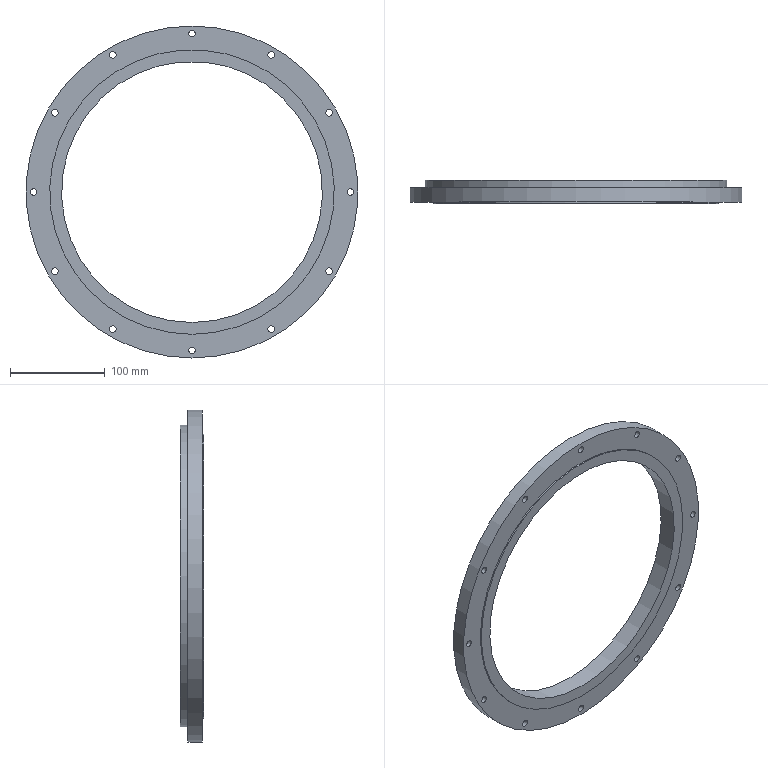Part | STEP file | Part [24] | 1 solid | 48 faces | box 350 x 24.5 x 350 mm | volume 570705 mm3 | cylinder 30 | plane 18 | commonest cylinder face diameters 7 x12 12 x12 275 x1 290 x1 300 x1 310 x1
STEP:
#1=CARTESIAN_POINT('',(0.,16.5,-175.));
#2=VERTEX_POINT('',#1);
#3=CARTESIAN_POINT('',(0.,16.5,0.));
#4=DIRECTION('',(0.,-1.,0.));
#5=DIRECTION('',(0.,0.,-1.));
#6=AXIS2_PLACEMENT_3D('',#3,#4,#5);
#7=CIRCLE('',#6,175.);
#8=EDGE_CURVE('',#2,#2,#7,.T.);
#9=ORIENTED_EDGE('',*,*,#8,.F.);
#10=EDGE_LOOP('',(#9));
#11=FACE_BOUND('',#10,.T.);
#12=CARTESIAN_POINT('',(88.696,16.5,141.626));
#13=VERTEX_POINT('',#12);
#14=CARTESIAN_POINT('',(83.5,16.5,144.626));
#15=DIRECTION('',(0.,1.,0.));
#16=DIRECTION('',(0.866,0.,-0.5));
#17=AXIS2_PLACEMENT_3D('',#14,#15,#16);
#18=CIRCLE('',#17,6.);
#19=EDGE_CURVE('',#13,#13,#18,.F.);
#20=ORIENTED_EDGE('',*,*,#19,.T.);
#21=EDGE_LOOP('',(#20));
#22=FACE_BOUND('',#21,.T.);
#23=CARTESIAN_POINT('',(147.626,16.5,78.304));
#24=VERTEX_POINT('',#23);
#25=CARTESIAN_POINT('',(144.626,16.5,83.5));
#26=DIRECTION('',(0.,1.,0.));
#27=DIRECTION('',(0.5,0.,-0.866));
#28=AXIS2_PLACEMENT_3D('',#25,#26,#27);
#29=CIRCLE('',#28,6.);
#30=EDGE_CURVE('',#24,#24,#29,.F.);
#31=ORIENTED_EDGE('',*,*,#30,.T.);
#32=EDGE_LOOP('',(#31));
#33=FACE_BOUND('',#32,.T.);
#34=CARTESIAN_POINT('',(167.,16.5,-6.));
#35=VERTEX_POINT('',#34);
#36=CARTESIAN_POINT('',(167.,16.5,0.));
#37=DIRECTION('',(0.,1.,0.));
#38=DIRECTION('',(0.,0.,-1.));
#39=AXIS2_PLACEMENT_3D('',#36,#37,#38);
#40=CIRCLE('',#39,6.);
#41=EDGE_CURVE('',#35,#35,#40,.F.);
#42=ORIENTED_EDGE('',*,*,#41,.T.);
#43=EDGE_LOOP('',(#42));
#44=FACE_BOUND('',#43,.T.);
#45=CARTESIAN_POINT('',(141.626,16.5,-88.696));
#46=VERTEX_POINT('',#45);
#47=CARTESIAN_POINT('',(144.626,16.5,-83.5));
#48=DIRECTION('',(0.,1.,0.));
#49=DIRECTION('',(-0.5,0.,-0.866));
#50=AXIS2_PLACEMENT_3D('',#47,#48,#49);
#51=CIRCLE('',#50,6.);
#52=EDGE_CURVE('',#46,#46,#51,.F.);
#53=ORIENTED_EDGE('',*,*,#52,.T.);
#54=EDGE_LOOP('',(#53));
#55=FACE_BOUND('',#54,.T.);
#56=CARTESIAN_POINT('',(78.304,16.5,-147.626));
#57=VERTEX_POINT('',#56);
#58=CARTESIAN_POINT('',(83.5,16.5,-144.626));
#59=DIRECTION('',(0.,1.,0.));
#60=DIRECTION('',(-0.866,0.,-0.5));
#61=AXIS2_PLACEMENT_3D('',#58,#59,#60);
#62=CIRCLE('',#61,6.);
#63=EDGE_CURVE('',#57,#57,#62,.F.);
#64=ORIENTED_EDGE('',*,*,#63,.T.);
#65=EDGE_LOOP('',(#64));
#66=FACE_BOUND('',#65,.T.);
#67=CARTESIAN_POINT('',(-6.,16.5,-167.));
#68=VERTEX_POINT('',#67);
#69=CARTESIAN_POINT('',(0.,16.5,-167.));
#70=DIRECTION('',(0.,1.,0.));
#71=DIRECTION('',(-1.,0.,0.));
#72=AXIS2_PLACEMENT_3D('',#69,#70,#71);
#73=CIRCLE('',#72,6.);
#74=EDGE_CURVE('',#68,#68,#73,.F.);
#75=ORIENTED_EDGE('',*,*,#74,.T.);
#76=EDGE_LOOP('',(#75));
#77=FACE_BOUND('',#76,.T.);
#78=CARTESIAN_POINT('',(-88.696,16.5,-141.626));
#79=VERTEX_POINT('',#78);
#80=CARTESIAN_POINT('',(-83.5,16.5,-144.626));
#81=DIRECTION('',(0.,1.,0.));
#82=DIRECTION('',(-0.866,0.,0.5));
#83=AXIS2_PLACEMENT_3D('',#80,#81,#82);
#84=CIRCLE('',#83,6.);
#85=EDGE_CURVE('',#79,#79,#84,.F.);
#86=ORIENTED_EDGE('',*,*,#85,.T.);
#87=EDGE_LOOP('',(#86));
#88=FACE_BOUND('',#87,.T.);
#89=CARTESIAN_POINT('',(-147.626,16.5,-78.304));
#90=VERTEX_POINT('',#89);
#91=CARTESIAN_POINT('',(-144.626,16.5,-83.5));
#92=DIRECTION('',(0.,1.,0.));
#93=DIRECTION('',(-0.5,0.,0.866));
#94=AXIS2_PLACEMENT_3D('',#91,#92,#93);
#95=CIRCLE('',#94,6.);
#96=EDGE_CURVE('',#90,#90,#95,.F.);
#97=ORIENTED_EDGE('',*,*,#96,.T.);
#98=EDGE_LOOP('',(#97));
#99=FACE_BOUND('',#98,.T.);
#100=CARTESIAN_POINT('',(-167.,16.5,6.));
#101=VERTEX_POINT('',#100);
#102=CARTESIAN_POINT('',(-167.,16.5,0.));
#103=DIRECTION('',(0.,1.,0.));
#104=DIRECTION('',(0.,0.,1.));
#105=AXIS2_PLACEMENT_3D('',#102,#103,#104);
#106=CIRCLE('',#105,6.);
#107=EDGE_CURVE('',#101,#101,#106,.F.);
#108=ORIENTED_EDGE('',*,*,#107,.T.);
#109=EDGE_LOOP('',(#108));
#110=FACE_BOUND('',#109,.T.);
#111=CARTESIAN_POINT('',(-141.626,16.5,88.696));
#112=VERTEX_POINT('',#111);
#113=CARTESIAN_POINT('',(-144.626,16.5,83.5));
#114=DIRECTION('',(0.,1.,0.));
#115=DIRECTION('',(0.5,0.,0.866));
#116=AXIS2_PLACEMENT_3D('',#113,#114,#115);
#117=CIRCLE('',#116,6.);
#118=EDGE_CURVE('',#112,#112,#117,.F.);
#119=ORIENTED_EDGE('',*,*,#118,.T.);
#120=EDGE_LOOP('',(#119));
#121=FACE_BOUND('',#120,.T.);
#122=CARTESIAN_POINT('',(-78.304,16.5,147.626));
#123=VERTEX_POINT('',#122);
#124=CARTESIAN_POINT('',(-83.5,16.5,144.626));
#125=DIRECTION('',(0.,1.,0.));
#126=DIRECTION('',(0.866,0.,0.5));
#127=AXIS2_PLACEMENT_3D('',#124,#125,#126);
#128=CIRCLE('',#127,6.);
#129=EDGE_CURVE('',#123,#123,#128,.F.);
#130=ORIENTED_EDGE('',*,*,#129,.T.);
#131=EDGE_LOOP('',(#130));
#132=FACE_BOUND('',#131,.T.);
#133=CARTESIAN_POINT('',(0.,16.5,-159.));
#134=VERTEX_POINT('',#133);
#135=CARTESIAN_POINT('',(0.,16.5,0.));
#136=DIRECTION('',(0.,-1.,0.));
#137=DIRECTION('',(0.,0.,-1.));
#138=AXIS2_PLACEMENT_3D('',#135,#136,#137);
#139=CIRCLE('',#138,159.);
#140=EDGE_CURVE('',#134,#134,#139,.T.);
#141=ORIENTED_EDGE('',*,*,#140,.T.);
#142=EDGE_LOOP('',(#141));
#143=FACE_BOUND('',#142,.T.);
#144=CARTESIAN_POINT('',(6.,16.5,167.));
#145=VERTEX_POINT('',#144);
#146=CARTESIAN_POINT('',(0.,16.5,167.));
#147=DIRECTION('',(0.,1.,0.));
#148=DIRECTION('',(1.,0.,0.));
#149=AXIS2_PLACEMENT_3D('',#146,#147,#148);
#150=CIRCLE('',#149,6.);
#151=EDGE_CURVE('',#145,#145,#150,.F.);
#152=ORIENTED_EDGE('',*,*,#151,.T.);
#153=EDGE_LOOP('',(#152));
#154=FACE_BOUND('',#153,.T.);
#155=CARTESIAN_POINT('',(0.,16.5,0.));
#156=DIRECTION('',(0.,1.,0.));
#157=DIRECTION('',(0.,0.,-1.));
#158=AXIS2_PLACEMENT_3D('',#155,#156,#157);
#159=PLANE('',#158);
#160=ADVANCED_FACE('',(#11,#22,#33,#44,#55,#66,#77,#88,#99,#110,#121,#132,#143,#154),#159,.T.);
#161=CARTESIAN_POINT('',(0.,1.5,-175.));
#162=VERTEX_POINT('',#161);
#163=CARTESIAN_POINT('',(0.,1.5,0.));
#164=DIRECTION('',(0.,-1.,0.));
#165=DIRECTION('',(0.,0.,-1.));
#166=AXIS2_PLACEMENT_3D('',#163,#164,#165);
#167=CIRCLE('',#166,175.);
#168=EDGE_CURVE('',#162,#162,#167,.T.);
#169=ORIENTED_EDGE('',*,*,#168,.T.);
#170=EDGE_LOOP('',(#169));
#171=FACE_BOUND('',#170,.T.);
#172=CARTESIAN_POINT('',(86.531,1.5,142.876));
#173=VERTEX_POINT('',#172);
#174=CARTESIAN_POINT('',(83.5,1.5,144.626));
#175=DIRECTION('',(0.,1.,0.));
#176=DIRECTION('',(0.866,0.,-0.5));
#177=AXIS2_PLACEMENT_3D('',#174,#175,#176);
#178=CIRCLE('',#177,3.5);
#179=EDGE_CURVE('',#173,#173,#178,.T.);
#180=ORIENTED_EDGE('',*,*,#179,.T.);
#181=EDGE_LOOP('',(#180));
#182=FACE_BOUND('',#181,.T.);
#183=CARTESIAN_POINT('',(146.376,1.5,80.469));
#184=VERTEX_POINT('',#183);
#185=CARTESIAN_POINT('',(144.626,1.5,83.5));
#186=DIRECTION('',(0.,1.,0.));
#187=DIRECTION('',(0.5,0.,-0.866));
#188=AXIS2_PLACEMENT_3D('',#185,#186,#187);
#189=CIRCLE('',#188,3.5);
#190=EDGE_CURVE('',#184,#184,#189,.T.);
#191=ORIENTED_EDGE('',*,*,#190,.T.);
#192=EDGE_LOOP('',(#191));
#193=FACE_BOUND('',#192,.T.);
#194=CARTESIAN_POINT('',(167.,1.5,-3.5));
#195=VERTEX_POINT('',#194);
#196=CARTESIAN_POINT('',(167.,1.5,0.));
#197=DIRECTION('',(0.,1.,0.));
#198=DIRECTION('',(0.,0.,-1.));
#199=AXIS2_PLACEMENT_3D('',#196,#197,#198);
#200=CIRCLE('',#199,3.5);
#201=EDGE_CURVE('',#195,#195,#200,.T.);
#202=ORIENTED_EDGE('',*,*,#201,.T.);
#203=EDGE_LOOP('',(#202));
#204=FACE_BOUND('',#203,.T.);
#205=CARTESIAN_POINT('',(142.876,1.5,-86.531));
#206=VERTEX_POINT('',#205);
#207=CARTESIAN_POINT('',(144.626,1.5,-83.5));
#208=DIRECTION('',(0.,1.,0.));
#209=DIRECTION('',(-0.5,0.,-0.866));
#210=AXIS2_PLACEMENT_3D('',#207,#208,#209);
#211=CIRCLE('',#210,3.5);
#212=EDGE_CURVE('',#206,#206,#211,.T.);
#213=ORIENTED_EDGE('',*,*,#212,.T.);
#214=EDGE_LOOP('',(#213));
#215=FACE_BOUND('',#214,.T.);
#216=CARTESIAN_POINT('',(80.469,1.5,-146.376));
#217=VERTEX_POINT('',#216);
#218=CARTESIAN_POINT('',(83.5,1.5,-144.626));
#219=DIRECTION('',(0.,1.,0.));
#220=DIRECTION('',(-0.866,0.,-0.5));
#221=AXIS2_PLACEMENT_3D('',#218,#219,#220);
#222=CIRCLE('',#221,3.5);
#223=EDGE_CURVE('',#217,#217,#222,.T.);
#224=ORIENTED_EDGE('',*,*,#223,.T.);
#225=EDGE_LOOP('',(#224));
#226=FACE_BOUND('',#225,.T.);
#227=CARTESIAN_POINT('',(-3.5,1.5,-167.));
#228=VERTEX_POINT('',#227);
#229=CARTESIAN_POINT('',(0.,1.5,-167.));
#230=DIRECTION('',(0.,1.,0.));
#231=DIRECTION('',(-1.,0.,0.));
#232=AXIS2_PLACEMENT_3D('',#229,#230,#231);
#233=CIRCLE('',#232,3.5);
#234=EDGE_CURVE('',#228,#228,#233,.T.);
#235=ORIENTED_EDGE('',*,*,#234,.T.);
#236=EDGE_LOOP('',(#235));
#237=FACE_BOUND('',#236,.T.);
#238=CARTESIAN_POINT('',(-86.531,1.5,-142.876));
#239=VERTEX_POINT('',#238);
#240=CARTESIAN_POINT('',(-83.5,1.5,-144.626));
#241=DIRECTION('',(0.,1.,0.));
#242=DIRECTION('',(-0.866,0.,0.5));
#243=AXIS2_PLACEMENT_3D('',#240,#241,#242);
#244=CIRCLE('',#243,3.5);
#245=EDGE_CURVE('',#239,#239,#244,.T.);
#246=ORIENTED_EDGE('',*,*,#245,.T.);
#247=EDGE_LOOP('',(#246));
#248=FACE_BOUND('',#247,.T.);
#249=CARTESIAN_POINT('',(-146.376,1.5,-80.469));
#250=VERTEX_POINT('',#249);
#251=CARTESIAN_POINT('',(-144.626,1.5,-83.5));
#252=DIRECTION('',(0.,1.,0.));
#253=DIRECTION('',(-0.5,0.,0.866));
#254=AXIS2_PLACEMENT_3D('',#251,#252,#253);
#255=CIRCLE('',#254,3.5);
#256=EDGE_CURVE('',#250,#250,#255,.T.);
#257=ORIENTED_EDGE('',*,*,#256,.T.);
#258=EDGE_LOOP('',(#257));
#259=FACE_BOUND('',#258,.T.);
#260=CARTESIAN_POINT('',(-167.,1.5,3.5));
#261=VERTEX_POINT('',#260);
#262=CARTESIAN_POINT('',(-167.,1.5,0.));
#263=DIRECTION('',(0.,1.,0.));
#264=DIRECTION('',(0.,0.,1.));
#265=AXIS2_PLACEMENT_3D('',#262,#263,#264);
#266=CIRCLE('',#265,3.5);
#267=EDGE_CURVE('',#261,#261,#266,.T.);
#268=ORIENTED_EDGE('',*,*,#267,.T.);
#269=EDGE_LOOP('',(#268));
#270=FACE_BOUND('',#269,.T.);
#271=CARTESIAN_POINT('',(-142.876,1.5,86.531));
#272=VERTEX_POINT('',#271);
#273=CARTESIAN_POINT('',(-144.626,1.5,83.5));
#274=DIRECTION('',(0.,1.,0.));
#275=DIRECTION('',(0.5,0.,0.866));
#276=AXIS2_PLACEMENT_3D('',#273,#274,#275);
#277=CIRCLE('',#276,3.5);
#278=EDGE_CURVE('',#272,#272,#277,.T.);
#279=ORIENTED_EDGE('',*,*,#278,.T.);
#280=EDGE_LOOP('',(#279));
#281=FACE_BOUND('',#280,.T.);
#282=CARTESIAN_POINT('',(-80.469,1.5,146.376));
#283=VERTEX_POINT('',#282);
#284=CARTESIAN_POINT('',(-83.5,1.5,144.626));
#285=DIRECTION('',(0.,1.,0.));
#286=DIRECTION('',(0.866,0.,0.5));
#287=AXIS2_PLACEMENT_3D('',#284,#285,#286);
#288=CIRCLE('',#287,3.5);
#289=EDGE_CURVE('',#283,#283,#288,.T.);
#290=ORIENTED_EDGE('',*,*,#289,.T.);
#291=EDGE_LOOP('',(#290));
#292=FACE_BOUND('',#291,.T.);
#293=CARTESIAN_POINT('',(0.,1.5,-150.));
#294=VERTEX_POINT('',#293);
#295=CARTESIAN_POINT('',(0.,1.5,0.));
#296=DIRECTION('',(0.,-1.,0.));
#297=DIRECTION('',(0.,0.,-1.));
#298=AXIS2_PLACEMENT_3D('',#295,#296,#297);
#299=CIRCLE('',#298,150.);
#300=EDGE_CURVE('',#294,#294,#299,.T.);
#301=ORIENTED_EDGE('',*,*,#300,.F.);
#302=EDGE_LOOP('',(#301));
#303=FACE_BOUND('',#302,.T.);
#304=CARTESIAN_POINT('',(3.5,1.5,167.));
#305=VERTEX_POINT('',#304);
#306=CARTESIAN_POINT('',(0.,1.5,167.));
#307=DIRECTION('',(0.,1.,0.));
#308=DIRECTION('',(1.,0.,0.));
#309=AXIS2_PLACEMENT_3D('',#306,#307,#308);
#310=CIRCLE('',#309,3.5);
#311=EDGE_CURVE('',#305,#305,#310,.T.);
#312=ORIENTED_EDGE('',*,*,#311,.T.);
#313=EDGE_LOOP('',(#312));
#314=FACE_BOUND('',#313,.T.);
#315=CARTESIAN_POINT('',(0.,1.5,0.));
#316=DIRECTION('',(0.,-1.,0.));
#317=DIRECTION('',(0.,0.,-1.));
#318=AXIS2_PLACEMENT_3D('',#315,#316,#317);
#319=PLANE('',#318);
#320=ADVANCED_FACE('',(#171,#182,#193,#204,#215,#226,#237,#248,#259,#270,#281,#292,#303,#314),#319,.T.);
#321=CARTESIAN_POINT('',(-80.469,10.5,146.376));
#322=VERTEX_POINT('',#321);
#323=CARTESIAN_POINT('',(-83.5,10.5,144.626));
#324=DIRECTION('',(0.,1.,0.));
#325=DIRECTION('',(0.866,0.,0.5));
#326=AXIS2_PLACEMENT_3D('',#323,#324,#325);
#327=CIRCLE('',#326,3.5);
#328=EDGE_CURVE('',#322,#322,#327,.T.);
#329=ORIENTED_EDGE('',*,*,#328,.T.);
#330=EDGE_LOOP('',(#329));
#331=FACE_OUTER_BOUND('',#330,.T.);
#332=ORIENTED_EDGE('',*,*,#289,.F.);
#333=EDGE_LOOP('',(#332));
#334=FACE_OUTER_BOUND('',#333,.T.);
#335=CARTESIAN_POINT('',(-83.5,-23.5,144.626));
#336=DIRECTION('',(0.,1.,0.));
#337=DIRECTION('',(0.866,0.,0.5));
#338=AXIS2_PLACEMENT_3D('',#335,#336,#337);
#339=CYLINDRICAL_SURFACE('',#338,3.5);
#340=ADVANCED_FACE('',(#331,#334),#339,.F.);
#341=ORIENTED_EDGE('',*,*,#129,.F.);
#342=EDGE_LOOP('',(#341));
#343=FACE_OUTER_BOUND('',#342,.T.);
#344=CARTESIAN_POINT('',(-78.304,10.5,147.626));
#345=VERTEX_POINT('',#344);
#346=CARTESIAN_POINT('',(-83.5,10.5,144.626));
#347=DIRECTION('',(0.,1.,0.));
#348=DIRECTION('',(0.866,0.,0.5));
#349=AXIS2_PLACEMENT_3D('',#346,#347,#348);
#350=CIRCLE('',#349,6.);
#351=EDGE_CURVE('',#345,#345,#350,.T.);
#352=ORIENTED_EDGE('',*,*,#351,.F.);
#353=EDGE_LOOP('',(#352));
#354=FACE_OUTER_BOUND('',#353,.T.);
#355=CARTESIAN_POINT('',(-83.5,10.5,144.626));
#356=DIRECTION('',(0.,1.,0.));
#357=DIRECTION('',(0.866,0.,0.5));
#358=AXIS2_PLACEMENT_3D('',#355,#356,#357);
#359=CYLINDRICAL_SURFACE('',#358,6.);
#360=ADVANCED_FACE('',(#343,#354),#359,.F.);
#361=CARTESIAN_POINT('',(-142.876,10.5,86.531));
#362=VERTEX_POINT('',#361);
#363=CARTESIAN_POINT('',(-144.626,10.5,83.5));
#364=DIRECTION('',(0.,1.,0.));
#365=DIRECTION('',(0.5,0.,0.866));
#366=AXIS2_PLACEMENT_3D('',#363,#364,#365);
#367=CIRCLE('',#366,3.5);
#368=EDGE_CURVE('',#362,#362,#367,.T.);
#369=ORIENTED_EDGE('',*,*,#368,.T.);
#370=EDGE_LOOP('',(#369));
#371=FACE_OUTER_BOUND('',#370,.T.);
#372=ORIENTED_EDGE('',*,*,#278,.F.);
#373=EDGE_LOOP('',(#372));
#374=FACE_OUTER_BOUND('',#373,.T.);
#375=CARTESIAN_POINT('',(-144.626,-23.5,83.5));
#376=DIRECTION('',(0.,1.,0.));
#377=DIRECTION('',(0.5,0.,0.866));
#378=AXIS2_PLACEMENT_3D('',#375,#376,#377);
#379=CYLINDRICAL_SURFACE('',#378,3.5);
#380=ADVANCED_FACE('',(#371,#374),#379,.F.);
#381=ORIENTED_EDGE('',*,*,#118,.F.);
#382=EDGE_LOOP('',(#381));
#383=FACE_OUTER_BOUND('',#382,.T.);
#384=CARTESIAN_POINT('',(-141.626,10.5,88.696));
#385=VERTEX_POINT('',#384);
#386=CARTESIAN_POINT('',(-144.626,10.5,83.5));
#387=DIRECTION('',(0.,1.,0.));
#388=DIRECTION('',(0.5,0.,0.866));
#389=AXIS2_PLACEMENT_3D('',#386,#387,#388);
#390=CIRCLE('',#389,6.);
#391=EDGE_CURVE('',#385,#385,#390,.T.);
#392=ORIENTED_EDGE('',*,*,#391,.F.);
#393=EDGE_LOOP('',(#392));
#394=FACE_OUTER_BOUND('',#393,.T.);
#395=CARTESIAN_POINT('',(-144.626,10.5,83.5));
#396=DIRECTION('',(0.,1.,0.));
#397=DIRECTION('',(0.5,0.,0.866));
#398=AXIS2_PLACEMENT_3D('',#395,#396,#397);
#399=CYLINDRICAL_SURFACE('',#398,6.);
#400=ADVANCED_FACE('',(#383,#394),#399,.F.);
#401=CARTESIAN_POINT('',(-167.,10.5,3.5));
#402=VERTEX_POINT('',#401);
#403=CARTESIAN_POINT('',(-167.,10.5,0.));
#404=DIRECTION('',(0.,1.,0.));
#405=DIRECTION('',(0.,0.,1.));
#406=AXIS2_PLACEMENT_3D('',#403,#404,#405);
#407=CIRCLE('',#406,3.5);
#408=EDGE_CURVE('',#402,#402,#407,.T.);
#409=ORIENTED_EDGE('',*,*,#408,.T.);
#410=EDGE_LOOP('',(#409));
#411=FACE_OUTER_BOUND('',#410,.T.);
#412=ORIENTED_EDGE('',*,*,#267,.F.);
#413=EDGE_LOOP('',(#412));
#414=FACE_OUTER_BOUND('',#413,.T.);
#415=CARTESIAN_POINT('',(-167.,-23.5,0.));
#416=DIRECTION('',(0.,1.,0.));
#417=DIRECTION('',(0.,0.,1.));
#418=AXIS2_PLACEMENT_3D('',#415,#416,#417);
#419=CYLINDRICAL_SURFACE('',#418,3.5);
#420=ADVANCED_FACE('',(#411,#414),#419,.F.);
#421=ORIENTED_EDGE('',*,*,#107,.F.);
#422=EDGE_LOOP('',(#421));
#423=FACE_OUTER_BOUND('',#422,.T.);
#424=CARTESIAN_POINT('',(-167.,10.5,6.));
#425=VERTEX_POINT('',#424);
#426=CARTESIAN_POINT('',(-167.,10.5,0.));
#427=DIRECTION('',(0.,1.,0.));
#428=DIRECTION('',(0.,0.,1.));
#429=AXIS2_PLACEMENT_3D('',#426,#427,#428);
#430=CIRCLE('',#429,6.);
#431=EDGE_CURVE('',#425,#425,#430,.T.);
#432=ORIENTED_EDGE('',*,*,#431,.F.);
#433=EDGE_LOOP('',(#432));
#434=FACE_OUTER_BOUND('',#433,.T.);
#435=CARTESIAN_POINT('',(-167.,10.5,0.));
#436=DIRECTION('',(0.,1.,0.));
#437=DIRECTION('',(0.,0.,1.));
#438=AXIS2_PLACEMENT_3D('',#435,#436,#437);
#439=CYLINDRICAL_SURFACE('',#438,6.);
#440=ADVANCED_FACE('',(#423,#434),#439,.F.);
#441=CARTESIAN_POINT('',(-146.376,10.5,-80.469));
#442=VERTEX_POINT('',#441);
#443=CARTESIAN_POINT('',(-144.626,10.5,-83.5));
#444=DIRECTION('',(0.,1.,0.));
#445=DIRECTION('',(-0.5,0.,0.866));
#446=AXIS2_PLACEMENT_3D('',#443,#444,#445);
#447=CIRCLE('',#446,3.5);
#448=EDGE_CURVE('',#442,#442,#447,.T.);
#449=ORIENTED_EDGE('',*,*,#448,.T.);
#450=EDGE_LOOP('',(#449));
#451=FACE_OUTER_BOUND('',#450,.T.);
#452=ORIENTED_EDGE('',*,*,#256,.F.);
#453=EDGE_LOOP('',(#452));
#454=FACE_OUTER_BOUND('',#453,.T.);
#455=CARTESIAN_POINT('',(-144.626,-23.5,-83.5));
#456=DIRECTION('',(0.,1.,0.));
#457=DIRECTION('',(-0.5,0.,0.866));
#458=AXIS2_PLACEMENT_3D('',#455,#456,#457);
#459=CYLINDRICAL_SURFACE('',#458,3.5);
#460=ADVANCED_FACE('',(#451,#454),#459,.F.);
#461=ORIENTED_EDGE('',*,*,#96,.F.);
#462=EDGE_LOOP('',(#461));
#463=FACE_OUTER_BOUND('',#462,.T.);
#464=CARTESIAN_POINT('',(-147.626,10.5,-78.304));
#465=VERTEX_POINT('',#464);
#466=CARTESIAN_POINT('',(-144.626,10.5,-83.5));
#467=DIRECTION('',(0.,1.,0.));
#468=DIRECTION('',(-0.5,0.,0.866));
#469=AXIS2_PLACEMENT_3D('',#466,#467,#468);
#470=CIRCLE('',#469,6.);
#471=EDGE_CURVE('',#465,#465,#470,.T.);
#472=ORIENTED_EDGE('',*,*,#471,.F.);
#473=EDGE_LOOP('',(#472));
#474=FACE_OUTER_BOUND('',#473,.T.);
#475=CARTESIAN_POINT('',(-144.626,10.5,-83.5));
#476=DIRECTION('',(0.,1.,0.));
#477=DIRECTION('',(-0.5,0.,0.866));
#478=AXIS2_PLACEMENT_3D('',#475,#476,#477);
#479=CYLINDRICAL_SURFACE('',#478,6.);
#480=ADVANCED_FACE('',(#463,#474),#479,.F.);
#481=CARTESIAN_POINT('',(-86.531,10.5,-142.876));
#482=VERTEX_POINT('',#481);
#483=CARTESIAN_POINT('',(-83.5,10.5,-144.626));
#484=DIRECTION('',(0.,1.,0.));
#485=DIRECTION('',(-0.866,0.,0.5));
#486=AXIS2_PLACEMENT_3D('',#483,#484,#485);
#487=CIRCLE('',#486,3.5);
#488=EDGE_CURVE('',#482,#482,#487,.T.);
#489=ORIENTED_EDGE('',*,*,#488,.T.);
#490=EDGE_LOOP('',(#489));
#491=FACE_OUTER_BOUND('',#490,.T.);
#492=ORIENTED_EDGE('',*,*,#245,.F.);
#493=EDGE_LOOP('',(#492));
#494=FACE_OUTER_BOUND('',#493,.T.);
#495=CARTESIAN_POINT('',(-83.5,-23.5,-144.626));
#496=DIRECTION('',(0.,1.,0.));
#497=DIRECTION('',(-0.866,0.,0.5));
#498=AXIS2_PLACEMENT_3D('',#495,#496,#497);
#499=CYLINDRICAL_SURFACE('',#498,3.5);
#500=ADVANCED_FACE('',(#491,#494),#499,.F.);
#501=ORIENTED_EDGE('',*,*,#85,.F.);
#502=EDGE_LOOP('',(#501));
#503=FACE_OUTER_BOUND('',#502,.T.);
#504=CARTESIAN_POINT('',(-88.696,10.5,-141.626));
#505=VERTEX_POINT('',#504);
#506=CARTESIAN_POINT('',(-83.5,10.5,-144.626));
#507=DIRECTION('',(0.,1.,0.));
#508=DIRECTION('',(-0.866,0.,0.5));
#509=AXIS2_PLACEMENT_3D('',#506,#507,#508);
#510=CIRCLE('',#509,6.);
#511=EDGE_CURVE('',#505,#505,#510,.T.);
#512=ORIENTED_EDGE('',*,*,#511,.F.);
#513=EDGE_LOOP('',(#512));
#514=FACE_OUTER_BOUND('',#513,.T.);
#515=CARTESIAN_POINT('',(-83.5,10.5,-144.626));
#516=DIRECTION('',(0.,1.,0.));
#517=DIRECTION('',(-0.866,0.,0.5));
#518=AXIS2_PLACEMENT_3D('',#515,#516,#517);
#519=CYLINDRICAL_SURFACE('',#518,6.);
#520=ADVANCED_FACE('',(#503,#514),#519,.F.);
#521=CARTESIAN_POINT('',(-3.5,10.5,-167.));
#522=VERTEX_POINT('',#521);
#523=CARTESIAN_POINT('',(0.,10.5,-167.));
#524=DIRECTION('',(0.,1.,0.));
#525=DIRECTION('',(-1.,0.,0.));
#526=AXIS2_PLACEMENT_3D('',#523,#524,#525);
#527=CIRCLE('',#526,3.5);
#528=EDGE_CURVE('',#522,#522,#527,.T.);
#529=ORIENTED_EDGE('',*,*,#528,.T.);
#530=EDGE_LOOP('',(#529));
#531=FACE_OUTER_BOUND('',#530,.T.);
#532=ORIENTED_EDGE('',*,*,#234,.F.);
#533=EDGE_LOOP('',(#532));
#534=FACE_OUTER_BOUND('',#533,.T.);
#535=CARTESIAN_POINT('',(0.,-23.5,-167.));
#536=DIRECTION('',(0.,1.,0.));
#537=DIRECTION('',(-1.,0.,0.));
#538=AXIS2_PLACEMENT_3D('',#535,#536,#537);
#539=CYLINDRICAL_SURFACE('',#538,3.5);
#540=ADVANCED_FACE('',(#531,#534),#539,.F.);
#541=ORIENTED_EDGE('',*,*,#74,.F.);
#542=EDGE_LOOP('',(#541));
#543=FACE_OUTER_BOUND('',#542,.T.);
#544=CARTESIAN_POINT('',(-6.,10.5,-167.));
#545=VERTEX_POINT('',#544);
#546=CARTESIAN_POINT('',(0.,10.5,-167.));
#547=DIRECTION('',(0.,1.,0.));
#548=DIRECTION('',(-1.,0.,0.));
#549=AXIS2_PLACEMENT_3D('',#546,#547,#548);
#550=CIRCLE('',#549,6.);
#551=EDGE_CURVE('',#545,#545,#550,.T.);
#552=ORIENTED_EDGE('',*,*,#551,.F.);
#553=EDGE_LOOP('',(#552));
#554=FACE_OUTER_BOUND('',#553,.T.);
#555=CARTESIAN_POINT('',(0.,10.5,-167.));
#556=DIRECTION('',(0.,1.,0.));
#557=DIRECTION('',(-1.,0.,0.));
#558=AXIS2_PLACEMENT_3D('',#555,#556,#557);
#559=CYLINDRICAL_SURFACE('',#558,6.);
#560=ADVANCED_FACE('',(#543,#554),#559,.F.);
#561=CARTESIAN_POINT('',(80.469,10.5,-146.376));
#562=VERTEX_POINT('',#561);
#563=CARTESIAN_POINT('',(83.5,10.5,-144.626));
#564=DIRECTION('',(0.,1.,0.));
#565=DIRECTION('',(-0.866,0.,-0.5));
#566=AXIS2_PLACEMENT_3D('',#563,#564,#565);
#567=CIRCLE('',#566,3.5);
#568=EDGE_CURVE('',#562,#562,#567,.T.);
#569=ORIENTED_EDGE('',*,*,#568,.T.);
#570=EDGE_LOOP('',(#569));
#571=FACE_OUTER_BOUND('',#570,.T.);
#572=ORIENTED_EDGE('',*,*,#223,.F.);
#573=EDGE_LOOP('',(#572));
#574=FACE_OUTER_BOUND('',#573,.T.);
#575=CARTESIAN_POINT('',(83.5,-23.5,-144.626));
#576=DIRECTION('',(0.,1.,0.));
#577=DIRECTION('',(-0.866,0.,-0.5));
#578=AXIS2_PLACEMENT_3D('',#575,#576,#577);
#579=CYLINDRICAL_SURFACE('',#578,3.5);
#580=ADVANCED_FACE('',(#571,#574),#579,.F.);
#581=ORIENTED_EDGE('',*,*,#63,.F.);
#582=EDGE_LOOP('',(#581));
#583=FACE_OUTER_BOUND('',#582,.T.);
#584=CARTESIAN_POINT('',(78.304,10.5,-147.626));
#585=VERTEX_POINT('',#584);
#586=CARTESIAN_POINT('',(83.5,10.5,-144.626));
#587=DIRECTION('',(0.,1.,0.));
#588=DIRECTION('',(-0.866,0.,-0.5));
#589=AXIS2_PLACEMENT_3D('',#586,#587,#588);
#590=CIRCLE('',#589,6.);
#591=EDGE_CURVE('',#585,#585,#590,.T.);
#592=ORIENTED_EDGE('',*,*,#591,.F.);
#593=EDGE_LOOP('',(#592));
#594=FACE_OUTER_BOUND('',#593,.T.);
#595=CARTESIAN_POINT('',(83.5,10.5,-144.626));
#596=DIRECTION('',(0.,1.,0.));
#597=DIRECTION('',(-0.866,0.,-0.5));
#598=AXIS2_PLACEMENT_3D('',#595,#596,#597);
#599=CYLINDRICAL_SURFACE('',#598,6.);
#600=ADVANCED_FACE('',(#583,#594),#599,.F.);
#601=CARTESIAN_POINT('',(142.876,10.5,-86.531));
#602=VERTEX_POINT('',#601);
#603=CARTESIAN_POINT('',(144.626,10.5,-83.5));
#604=DIRECTION('',(0.,1.,0.));
#605=DIRECTION('',(-0.5,0.,-0.866));
#606=AXIS2_PLACEMENT_3D('',#603,#604,#605);
#607=CIRCLE('',#606,3.5);
#608=EDGE_CURVE('',#602,#602,#607,.T.);
#609=ORIENTED_EDGE('',*,*,#608,.T.);
#610=EDGE_LOOP('',(#609));
#611=FACE_OUTER_BOUND('',#610,.T.);
#612=ORIENTED_EDGE('',*,*,#212,.F.);
#613=EDGE_LOOP('',(#612));
#614=FACE_OUTER_BOUND('',#613,.T.);
#615=CARTESIAN_POINT('',(144.626,-23.5,-83.5));
#616=DIRECTION('',(0.,1.,0.));
#617=DIRECTION('',(-0.5,0.,-0.866));
#618=AXIS2_PLACEMENT_3D('',#615,#616,#617);
#619=CYLINDRICAL_SURFACE('',#618,3.5);
#620=ADVANCED_FACE('',(#611,#614),#619,.F.);
#621=ORIENTED_EDGE('',*,*,#52,.F.);
#622=EDGE_LOOP('',(#621));
#623=FACE_OUTER_BOUND('',#622,.T.);
#624=CARTESIAN_POINT('',(141.626,10.5,-88.696));
#625=VERTEX_POINT('',#624);
#626=CARTESIAN_POINT('',(144.626,10.5,-83.5));
#627=DIRECTION('',(0.,1.,0.));
#628=DIRECTION('',(-0.5,0.,-0.866));
#629=AXIS2_PLACEMENT_3D('',#626,#627,#628);
#630=CIRCLE('',#629,6.);
#631=EDGE_CURVE('',#625,#625,#630,.T.);
#632=ORIENTED_EDGE('',*,*,#631,.F.);
#633=EDGE_LOOP('',(#632));
#634=FACE_OUTER_BOUND('',#633,.T.);
#635=CARTESIAN_POINT('',(144.626,10.5,-83.5));
#636=DIRECTION('',(0.,1.,0.));
#637=DIRECTION('',(-0.5,0.,-0.866));
#638=AXIS2_PLACEMENT_3D('',#635,#636,#637);
#639=CYLINDRICAL_SURFACE('',#638,6.);
#640=ADVANCED_FACE('',(#623,#634),#639,.F.);
#641=CARTESIAN_POINT('',(167.,10.5,-3.5));
#642=VERTEX_POINT('',#641);
#643=CARTESIAN_POINT('',(167.,10.5,0.));
#644=DIRECTION('',(0.,1.,0.));
#645=DIRECTION('',(0.,0.,-1.));
#646=AXIS2_PLACEMENT_3D('',#643,#644,#645);
#647=CIRCLE('',#646,3.5);
#648=EDGE_CURVE('',#642,#642,#647,.T.);
#649=ORIENTED_EDGE('',*,*,#648,.T.);
#650=EDGE_LOOP('',(#649));
#651=FACE_OUTER_BOUND('',#650,.T.);
#652=ORIENTED_EDGE('',*,*,#201,.F.);
#653=EDGE_LOOP('',(#652));
#654=FACE_OUTER_BOUND('',#653,.T.);
#655=CARTESIAN_POINT('',(167.,-23.5,0.));
#656=DIRECTION('',(0.,1.,0.));
#657=DIRECTION('',(0.,0.,-1.));
#658=AXIS2_PLACEMENT_3D('',#655,#656,#657);
#659=CYLINDRICAL_SURFACE('',#658,3.5);
#660=ADVANCED_FACE('',(#651,#654),#659,.F.);
#661=ORIENTED_EDGE('',*,*,#41,.F.);
#662=EDGE_LOOP('',(#661));
#663=FACE_OUTER_BOUND('',#662,.T.);
#664=CARTESIAN_POINT('',(167.,10.5,-6.));
#665=VERTEX_POINT('',#664);
#666=CARTESIAN_POINT('',(167.,10.5,0.));
#667=DIRECTION('',(0.,1.,0.));
#668=DIRECTION('',(0.,0.,-1.));
#669=AXIS2_PLACEMENT_3D('',#666,#667,#668);
#670=CIRCLE('',#669,6.);
#671=EDGE_CURVE('',#665,#665,#670,.T.);
#672=ORIENTED_EDGE('',*,*,#671,.F.);
#673=EDGE_LOOP('',(#672));
#674=FACE_OUTER_BOUND('',#673,.T.);
#675=CARTESIAN_POINT('',(167.,10.5,0.));
#676=DIRECTION('',(0.,1.,0.));
#677=DIRECTION('',(0.,0.,-1.));
#678=AXIS2_PLACEMENT_3D('',#675,#676,#677);
#679=CYLINDRICAL_SURFACE('',#678,6.);
#680=ADVANCED_FACE('',(#663,#674),#679,.F.);
#681=CARTESIAN_POINT('',(146.376,10.5,80.469));
#682=VERTEX_POINT('',#681);
#683=CARTESIAN_POINT('',(144.626,10.5,83.5));
#684=DIRECTION('',(0.,1.,0.));
#685=DIRECTION('',(0.5,0.,-0.866));
#686=AXIS2_PLACEMENT_3D('',#683,#684,#685);
#687=CIRCLE('',#686,3.5);
#688=EDGE_CURVE('',#682,#682,#687,.T.);
#689=ORIENTED_EDGE('',*,*,#688,.T.);
#690=EDGE_LOOP('',(#689));
#691=FACE_OUTER_BOUND('',#690,.T.);
#692=ORIENTED_EDGE('',*,*,#190,.F.);
#693=EDGE_LOOP('',(#692));
#694=FACE_OUTER_BOUND('',#693,.T.);
#695=CARTESIAN_POINT('',(144.626,-23.5,83.5));
#696=DIRECTION('',(0.,1.,0.));
#697=DIRECTION('',(0.5,0.,-0.866));
#698=AXIS2_PLACEMENT_3D('',#695,#696,#697);
#699=CYLINDRICAL_SURFACE('',#698,3.5);
#700=ADVANCED_FACE('',(#691,#694),#699,.F.);
#701=ORIENTED_EDGE('',*,*,#30,.F.);
#702=EDGE_LOOP('',(#701));
#703=FACE_OUTER_BOUND('',#702,.T.);
#704=CARTESIAN_POINT('',(147.626,10.5,78.304));
#705=VERTEX_POINT('',#704);
#706=CARTESIAN_POINT('',(144.626,10.5,83.5));
#707=DIRECTION('',(0.,1.,0.));
#708=DIRECTION('',(0.5,0.,-0.866));
#709=AXIS2_PLACEMENT_3D('',#706,#707,#708);
#710=CIRCLE('',#709,6.);
#711=EDGE_CURVE('',#705,#705,#710,.T.);
#712=ORIENTED_EDGE('',*,*,#711,.F.);
#713=EDGE_LOOP('',(#712));
#714=FACE_OUTER_BOUND('',#713,.T.);
#715=CARTESIAN_POINT('',(144.626,10.5,83.5));
#716=DIRECTION('',(0.,1.,0.));
#717=DIRECTION('',(0.5,0.,-0.866));
#718=AXIS2_PLACEMENT_3D('',#715,#716,#717);
#719=CYLINDRICAL_SURFACE('',#718,6.);
#720=ADVANCED_FACE('',(#703,#714),#719,.F.);
#721=CARTESIAN_POINT('',(86.531,10.5,142.876));
#722=VERTEX_POINT('',#721);
#723=CARTESIAN_POINT('',(83.5,10.5,144.626));
#724=DIRECTION('',(0.,1.,0.));
#725=DIRECTION('',(0.866,0.,-0.5));
#726=AXIS2_PLACEMENT_3D('',#723,#724,#725);
#727=CIRCLE('',#726,3.5);
#728=EDGE_CURVE('',#722,#722,#727,.T.);
#729=ORIENTED_EDGE('',*,*,#728,.T.);
#730=EDGE_LOOP('',(#729));
#731=FACE_OUTER_BOUND('',#730,.T.);
#732=ORIENTED_EDGE('',*,*,#179,.F.);
#733=EDGE_LOOP('',(#732));
#734=FACE_OUTER_BOUND('',#733,.T.);
#735=CARTESIAN_POINT('',(83.5,-23.5,144.626));
#736=DIRECTION('',(0.,1.,0.));
#737=DIRECTION('',(0.866,0.,-0.5));
#738=AXIS2_PLACEMENT_3D('',#735,#736,#737);
#739=CYLINDRICAL_SURFACE('',#738,3.5);
#740=ADVANCED_FACE('',(#731,#734),#739,.F.);
#741=ORIENTED_EDGE('',*,*,#19,.F.);
#742=EDGE_LOOP('',(#741));
#743=FACE_OUTER_BOUND('',#742,.T.);
#744=CARTESIAN_POINT('',(88.696,10.5,141.626));
#745=VERTEX_POINT('',#744);
#746=CARTESIAN_POINT('',(83.5,10.5,144.626));
#747=DIRECTION('',(0.,1.,0.));
#748=DIRECTION('',(0.866,0.,-0.5));
#749=AXIS2_PLACEMENT_3D('',#746,#747,#748);
#750=CIRCLE('',#749,6.);
#751=EDGE_CURVE('',#745,#745,#750,.T.);
#752=ORIENTED_EDGE('',*,*,#751,.F.);
#753=EDGE_LOOP('',(#752));
#754=FACE_OUTER_BOUND('',#753,.T.);
#755=CARTESIAN_POINT('',(83.5,10.5,144.626));
#756=DIRECTION('',(0.,1.,0.));
#757=DIRECTION('',(0.866,0.,-0.5));
#758=AXIS2_PLACEMENT_3D('',#755,#756,#757);
#759=CYLINDRICAL_SURFACE('',#758,6.);
#760=ADVANCED_FACE('',(#743,#754),#759,.F.);
#761=ORIENTED_EDGE('',*,*,#8,.T.);
#762=EDGE_LOOP('',(#761));
#763=FACE_OUTER_BOUND('',#762,.T.);
#764=ORIENTED_EDGE('',*,*,#168,.F.);
#765=EDGE_LOOP('',(#764));
#766=FACE_OUTER_BOUND('',#765,.T.);
#767=CARTESIAN_POINT('',(0.,16.5,0.));
#768=DIRECTION('',(0.,-1.,0.));
#769=DIRECTION('',(0.,0.,-1.));
#770=AXIS2_PLACEMENT_3D('',#767,#768,#769);
#771=CYLINDRICAL_SURFACE('',#770,175.);
#772=ADVANCED_FACE('',(#763,#766),#771,.T.);
#773=CARTESIAN_POINT('',(0.,24.5,-159.));
#774=VERTEX_POINT('',#773);
#775=CARTESIAN_POINT('',(0.,24.5,0.));
#776=DIRECTION('',(0.,-1.,0.));
#777=DIRECTION('',(0.,0.,-1.));
#778=AXIS2_PLACEMENT_3D('',#775,#776,#777);
#779=CIRCLE('',#778,159.);
#780=EDGE_CURVE('',#774,#774,#779,.T.);
#781=ORIENTED_EDGE('',*,*,#780,.T.);
#782=EDGE_LOOP('',(#781));
#783=FACE_OUTER_BOUND('',#782,.T.);
#784=ORIENTED_EDGE('',*,*,#140,.F.);
#785=EDGE_LOOP('',(#784));
#786=FACE_OUTER_BOUND('',#785,.T.);
#787=CARTESIAN_POINT('',(0.,24.5,0.));
#788=DIRECTION('',(0.,-1.,0.));
#789=DIRECTION('',(0.,0.,-1.));
#790=AXIS2_PLACEMENT_3D('',#787,#788,#789);
#791=CYLINDRICAL_SURFACE('',#790,159.);
#792=ADVANCED_FACE('',(#783,#786),#791,.T.);
#793=ORIENTED_EDGE('',*,*,#151,.F.);
#794=EDGE_LOOP('',(#793));
#795=FACE_OUTER_BOUND('',#794,.T.);
#796=CARTESIAN_POINT('',(6.,10.5,167.));
#797=VERTEX_POINT('',#796);
#798=CARTESIAN_POINT('',(0.,10.5,167.));
#799=DIRECTION('',(0.,1.,0.));
#800=DIRECTION('',(1.,0.,0.));
#801=AXIS2_PLACEMENT_3D('',#798,#799,#800);
#802=CIRCLE('',#801,6.);
#803=EDGE_CURVE('',#797,#797,#802,.T.);
#804=ORIENTED_EDGE('',*,*,#803,.F.);
#805=EDGE_LOOP('',(#804));
#806=FACE_OUTER_BOUND('',#805,.T.);
#807=CARTESIAN_POINT('',(0.,10.5,167.));
#808=DIRECTION('',(0.,1.,0.));
#809=DIRECTION('',(1.,0.,0.));
#810=AXIS2_PLACEMENT_3D('',#807,#808,#809);
#811=CYLINDRICAL_SURFACE('',#810,6.);
#812=ADVANCED_FACE('',(#795,#806),#811,.F.);
#813=ORIENTED_EDGE('',*,*,#300,.T.);
#814=EDGE_LOOP('',(#813));
#815=FACE_OUTER_BOUND('',#814,.T.);
#816=CARTESIAN_POINT('',(0.,0.,-150.));
#817=VERTEX_POINT('',#816);
#818=CARTESIAN_POINT('',(0.,0.,0.));
#819=DIRECTION('',(0.,-1.,0.));
#820=DIRECTION('',(0.,0.,-1.));
#821=AXIS2_PLACEMENT_3D('',#818,#819,#820);
#822=CIRCLE('',#821,150.);
#823=EDGE_CURVE('',#817,#817,#822,.T.);
#824=ORIENTED_EDGE('',*,*,#823,.F.);
#825=EDGE_LOOP('',(#824));
#826=FACE_OUTER_BOUND('',#825,.T.);
#827=CARTESIAN_POINT('',(0.,1.5,0.));
#828=DIRECTION('',(0.,-1.,0.));
#829=DIRECTION('',(0.,0.,-1.));
#830=AXIS2_PLACEMENT_3D('',#827,#828,#829);
#831=CYLINDRICAL_SURFACE('',#830,150.);
#832=ADVANCED_FACE('',(#815,#826),#831,.T.);
#833=CARTESIAN_POINT('',(3.5,10.5,167.));
#834=VERTEX_POINT('',#833);
#835=CARTESIAN_POINT('',(0.,10.5,167.));
#836=DIRECTION('',(0.,1.,0.));
#837=DIRECTION('',(1.,0.,0.));
#838=AXIS2_PLACEMENT_3D('',#835,#836,#837);
#839=CIRCLE('',#838,3.5);
#840=EDGE_CURVE('',#834,#834,#839,.T.);
#841=ORIENTED_EDGE('',*,*,#840,.T.);
#842=EDGE_LOOP('',(#841));
#843=FACE_OUTER_BOUND('',#842,.T.);
#844=ORIENTED_EDGE('',*,*,#311,.F.);
#845=EDGE_LOOP('',(#844));
#846=FACE_OUTER_BOUND('',#845,.T.);
#847=CARTESIAN_POINT('',(0.,-23.5,167.));
#848=DIRECTION('',(0.,1.,0.));
#849=DIRECTION('',(1.,0.,0.));
#850=AXIS2_PLACEMENT_3D('',#847,#848,#849);
#851=CYLINDRICAL_SURFACE('',#850,3.5);
#852=ADVANCED_FACE('',(#843,#846),#851,.F.);
#853=ORIENTED_EDGE('',*,*,#351,.T.);
#854=EDGE_LOOP('',(#853));
#855=FACE_BOUND('',#854,.T.);
#856=ORIENTED_EDGE('',*,*,#328,.F.);
#857=EDGE_LOOP('',(#856));
#858=FACE_BOUND('',#857,.T.);
#859=CARTESIAN_POINT('',(-83.5,10.5,144.626));
#860=DIRECTION('',(0.,-1.,0.));
#861=DIRECTION('',(0.866,0.,0.5));
#862=AXIS2_PLACEMENT_3D('',#859,#860,#861);
#863=PLANE('',#862);
#864=ADVANCED_FACE('',(#855,#858),#863,.F.);
#865=ORIENTED_EDGE('',*,*,#391,.T.);
#866=EDGE_LOOP('',(#865));
#867=FACE_BOUND('',#866,.T.);
#868=ORIENTED_EDGE('',*,*,#368,.F.);
#869=EDGE_LOOP('',(#868));
#870=FACE_BOUND('',#869,.T.);
#871=CARTESIAN_POINT('',(-144.626,10.5,83.5));
#872=DIRECTION('',(0.,-1.,0.));
#873=DIRECTION('',(0.5,0.,0.866));
#874=AXIS2_PLACEMENT_3D('',#871,#872,#873);
#875=PLANE('',#874);
#876=ADVANCED_FACE('',(#867,#870),#875,.F.);
#877=ORIENTED_EDGE('',*,*,#431,.T.);
#878=EDGE_LOOP('',(#877));
#879=FACE_BOUND('',#878,.T.);
#880=ORIENTED_EDGE('',*,*,#408,.F.);
#881=EDGE_LOOP('',(#880));
#882=FACE_BOUND('',#881,.T.);
#883=CARTESIAN_POINT('',(-167.,10.5,0.));
#884=DIRECTION('',(0.,-1.,0.));
#885=DIRECTION('',(0.,0.,1.));
#886=AXIS2_PLACEMENT_3D('',#883,#884,#885);
#887=PLANE('',#886);
#888=ADVANCED_FACE('',(#879,#882),#887,.F.);
#889=ORIENTED_EDGE('',*,*,#471,.T.);
#890=EDGE_LOOP('',(#889));
#891=FACE_BOUND('',#890,.T.);
#892=ORIENTED_EDGE('',*,*,#448,.F.);
#893=EDGE_LOOP('',(#892));
#894=FACE_BOUND('',#893,.T.);
#895=CARTESIAN_POINT('',(-144.626,10.5,-83.5));
#896=DIRECTION('',(0.,-1.,0.));
#897=DIRECTION('',(-0.5,0.,0.866));
#898=AXIS2_PLACEMENT_3D('',#895,#896,#897);
#899=PLANE('',#898);
#900=ADVANCED_FACE('',(#891,#894),#899,.F.);
#901=ORIENTED_EDGE('',*,*,#511,.T.);
#902=EDGE_LOOP('',(#901));
#903=FACE_BOUND('',#902,.T.);
#904=ORIENTED_EDGE('',*,*,#488,.F.);
#905=EDGE_LOOP('',(#904));
#906=FACE_BOUND('',#905,.T.);
#907=CARTESIAN_POINT('',(-83.5,10.5,-144.626));
#908=DIRECTION('',(0.,-1.,0.));
#909=DIRECTION('',(-0.866,0.,0.5));
#910=AXIS2_PLACEMENT_3D('',#907,#908,#909);
#911=PLANE('',#910);
#912=ADVANCED_FACE('',(#903,#906),#911,.F.);
#913=ORIENTED_EDGE('',*,*,#551,.T.);
#914=EDGE_LOOP('',(#913));
#915=FACE_BOUND('',#914,.T.);
#916=ORIENTED_EDGE('',*,*,#528,.F.);
#917=EDGE_LOOP('',(#916));
#918=FACE_BOUND('',#917,.T.);
#919=CARTESIAN_POINT('',(0.,10.5,-167.));
#920=DIRECTION('',(0.,-1.,0.));
#921=DIRECTION('',(-1.,0.,0.));
#922=AXIS2_PLACEMENT_3D('',#919,#920,#921);
#923=PLANE('',#922);
#924=ADVANCED_FACE('',(#915,#918),#923,.F.);
#925=ORIENTED_EDGE('',*,*,#591,.T.);
#926=EDGE_LOOP('',(#925));
#927=FACE_BOUND('',#926,.T.);
#928=ORIENTED_EDGE('',*,*,#568,.F.);
#929=EDGE_LOOP('',(#928));
#930=FACE_BOUND('',#929,.T.);
#931=CARTESIAN_POINT('',(83.5,10.5,-144.626));
#932=DIRECTION('',(0.,-1.,0.));
#933=DIRECTION('',(-0.866,0.,-0.5));
#934=AXIS2_PLACEMENT_3D('',#931,#932,#933);
#935=PLANE('',#934);
#936=ADVANCED_FACE('',(#927,#930),#935,.F.);
#937=ORIENTED_EDGE('',*,*,#631,.T.);
#938=EDGE_LOOP('',(#937));
#939=FACE_BOUND('',#938,.T.);
#940=ORIENTED_EDGE('',*,*,#608,.F.);
#941=EDGE_LOOP('',(#940));
#942=FACE_BOUND('',#941,.T.);
#943=CARTESIAN_POINT('',(144.626,10.5,-83.5));
#944=DIRECTION('',(0.,-1.,0.));
#945=DIRECTION('',(-0.5,0.,-0.866));
#946=AXIS2_PLACEMENT_3D('',#943,#944,#945);
#947=PLANE('',#946);
#948=ADVANCED_FACE('',(#939,#942),#947,.F.);
#949=ORIENTED_EDGE('',*,*,#671,.T.);
#950=EDGE_LOOP('',(#949));
#951=FACE_BOUND('',#950,.T.);
#952=ORIENTED_EDGE('',*,*,#648,.F.);
#953=EDGE_LOOP('',(#952));
#954=FACE_BOUND('',#953,.T.);
#955=CARTESIAN_POINT('',(167.,10.5,0.));
#956=DIRECTION('',(0.,-1.,0.));
#957=DIRECTION('',(0.,0.,-1.));
#958=AXIS2_PLACEMENT_3D('',#955,#956,#957);
#959=PLANE('',#958);
#960=ADVANCED_FACE('',(#951,#954),#959,.F.);
#961=ORIENTED_EDGE('',*,*,#711,.T.);
#962=EDGE_LOOP('',(#961));
#963=FACE_BOUND('',#962,.T.);
#964=ORIENTED_EDGE('',*,*,#688,.F.);
#965=EDGE_LOOP('',(#964));
#966=FACE_BOUND('',#965,.T.);
#967=CARTESIAN_POINT('',(144.626,10.5,83.5));
#968=DIRECTION('',(0.,-1.,0.));
#969=DIRECTION('',(0.5,0.,-0.866));
#970=AXIS2_PLACEMENT_3D('',#967,#968,#969);
#971=PLANE('',#970);
#972=ADVANCED_FACE('',(#963,#966),#971,.F.);
#973=ORIENTED_EDGE('',*,*,#751,.T.);
#974=EDGE_LOOP('',(#973));
#975=FACE_BOUND('',#974,.T.);
#976=ORIENTED_EDGE('',*,*,#728,.F.);
#977=EDGE_LOOP('',(#976));
#978=FACE_BOUND('',#977,.T.);
#979=CARTESIAN_POINT('',(83.5,10.5,144.626));
#980=DIRECTION('',(0.,-1.,0.));
#981=DIRECTION('',(0.866,0.,-0.5));
#982=AXIS2_PLACEMENT_3D('',#979,#980,#981);
#983=PLANE('',#982);
#984=ADVANCED_FACE('',(#975,#978),#983,.F.);
#985=ORIENTED_EDGE('',*,*,#780,.F.);
#986=EDGE_LOOP('',(#985));
#987=FACE_BOUND('',#986,.T.);
#988=CARTESIAN_POINT('',(0.,24.5,-155.));
#989=VERTEX_POINT('',#988);
#990=CARTESIAN_POINT('',(0.,24.5,0.));
#991=DIRECTION('',(0.,-1.,0.));
#992=DIRECTION('',(0.,0.,-1.));
#993=AXIS2_PLACEMENT_3D('',#990,#991,#992);
#994=CIRCLE('',#993,155.);
#995=EDGE_CURVE('',#989,#989,#994,.T.);
#996=ORIENTED_EDGE('',*,*,#995,.T.);
#997=EDGE_LOOP('',(#996));
#998=FACE_BOUND('',#997,.T.);
#999=CARTESIAN_POINT('',(0.,24.5,0.));
#1000=DIRECTION('',(0.,1.,0.));
#1001=DIRECTION('',(0.,0.,-1.));
#1002=AXIS2_PLACEMENT_3D('',#999,#1000,#1001);
#1003=PLANE('',#1002);
#1004=ADVANCED_FACE('',(#987,#998),#1003,.T.);
#1005=ORIENTED_EDGE('',*,*,#803,.T.);
#1006=EDGE_LOOP('',(#1005));
#1007=FACE_BOUND('',#1006,.T.);
#1008=ORIENTED_EDGE('',*,*,#840,.F.);
#1009=EDGE_LOOP('',(#1008));
#1010=FACE_BOUND('',#1009,.T.);
#1011=CARTESIAN_POINT('',(0.,10.5,167.));
#1012=DIRECTION('',(0.,-1.,0.));
#1013=DIRECTION('',(1.,0.,0.));
#1014=AXIS2_PLACEMENT_3D('',#1011,#1012,#1013);
#1015=PLANE('',#1014);
#1016=ADVANCED_FACE('',(#1007,#1010),#1015,.F.);
#1017=ORIENTED_EDGE('',*,*,#823,.T.);
#1018=EDGE_LOOP('',(#1017));
#1019=FACE_BOUND('',#1018,.T.);
#1020=CARTESIAN_POINT('',(0.,0.,-137.5));
#1021=VERTEX_POINT('',#1020);
#1022=CARTESIAN_POINT('',(0.,0.,0.));
#1023=DIRECTION('',(0.,-1.,0.));
#1024=DIRECTION('',(0.,0.,-1.));
#1025=AXIS2_PLACEMENT_3D('',#1022,#1023,#1024);
#1026=CIRCLE('',#1025,137.5);
#1027=EDGE_CURVE('',#1021,#1021,#1026,.T.);
#1028=ORIENTED_EDGE('',*,*,#1027,.F.);
#1029=EDGE_LOOP('',(#1028));
#1030=FACE_BOUND('',#1029,.T.);
#1031=CARTESIAN_POINT('',(0.,0.,0.));
#1032=DIRECTION('',(0.,-1.,0.));
#1033=DIRECTION('',(0.,0.,-1.));
#1034=AXIS2_PLACEMENT_3D('',#1031,#1032,#1033);
#1035=PLANE('',#1034);
#1036=ADVANCED_FACE('',(#1019,#1030),#1035,.T.);
#1037=ORIENTED_EDGE('',*,*,#995,.F.);
#1038=EDGE_LOOP('',(#1037));
#1039=FACE_OUTER_BOUND('',#1038,.T.);
#1040=CARTESIAN_POINT('',(0.,12.5,-155.));
#1041=VERTEX_POINT('',#1040);
#1042=CARTESIAN_POINT('',(0.,12.5,0.));
#1043=DIRECTION('',(0.,-1.,0.));
#1044=DIRECTION('',(0.,0.,-1.));
#1045=AXIS2_PLACEMENT_3D('',#1042,#1043,#1044);
#1046=CIRCLE('',#1045,155.);
#1047=EDGE_CURVE('',#1041,#1041,#1046,.T.);
#1048=ORIENTED_EDGE('',*,*,#1047,.T.);
#1049=EDGE_LOOP('',(#1048));
#1050=FACE_OUTER_BOUND('',#1049,.T.);
#1051=CARTESIAN_POINT('',(0.,12.5,0.));
#1052=DIRECTION('',(0.,-1.,0.));
#1053=DIRECTION('',(0.,0.,-1.));
#1054=AXIS2_PLACEMENT_3D('',#1051,#1052,#1053);
#1055=CYLINDRICAL_SURFACE('',#1054,155.);
#1056=ADVANCED_FACE('',(#1039,#1050),#1055,.F.);
#1057=CARTESIAN_POINT('',(0.,19.5,-137.5));
#1058=VERTEX_POINT('',#1057);
#1059=CARTESIAN_POINT('',(0.,19.5,0.));
#1060=DIRECTION('',(0.,-1.,0.));
#1061=DIRECTION('',(0.,0.,-1.));
#1062=AXIS2_PLACEMENT_3D('',#1059,#1060,#1061);
#1063=CIRCLE('',#1062,137.5);
#1064=EDGE_CURVE('',#1058,#1058,#1063,.T.);
#1065=ORIENTED_EDGE('',*,*,#1064,.F.);
#1066=EDGE_LOOP('',(#1065));
#1067=FACE_OUTER_BOUND('',#1066,.T.);
#1068=ORIENTED_EDGE('',*,*,#1027,.T.);
#1069=EDGE_LOOP('',(#1068));
#1070=FACE_OUTER_BOUND('',#1069,.T.);
#1071=CARTESIAN_POINT('',(0.,0.,0.));
#1072=DIRECTION('',(0.,-1.,0.));
#1073=DIRECTION('',(0.,0.,-1.));
#1074=AXIS2_PLACEMENT_3D('',#1071,#1072,#1073);
#1075=CYLINDRICAL_SURFACE('',#1074,137.5);
#1076=ADVANCED_FACE('',(#1067,#1070),#1075,.F.);
#1077=ORIENTED_EDGE('',*,*,#1047,.F.);
#1078=EDGE_LOOP('',(#1077));
#1079=FACE_BOUND('',#1078,.T.);
#1080=CARTESIAN_POINT('',(0.,12.5,-145.));
#1081=VERTEX_POINT('',#1080);
#1082=CARTESIAN_POINT('',(0.,12.5,0.));
#1083=DIRECTION('',(0.,-1.,0.));
#1084=DIRECTION('',(0.,0.,-1.));
#1085=AXIS2_PLACEMENT_3D('',#1082,#1083,#1084);
#1086=CIRCLE('',#1085,145.);
#1087=EDGE_CURVE('',#1081,#1081,#1086,.T.);
#1088=ORIENTED_EDGE('',*,*,#1087,.T.);
#1089=EDGE_LOOP('',(#1088));
#1090=FACE_BOUND('',#1089,.T.);
#1091=CARTESIAN_POINT('',(0.,12.5,0.));
#1092=DIRECTION('',(0.,1.,0.));
#1093=DIRECTION('',(0.,0.,-1.));
#1094=AXIS2_PLACEMENT_3D('',#1091,#1092,#1093);
#1095=PLANE('',#1094);
#1096=ADVANCED_FACE('',(#1079,#1090),#1095,.T.);
#1097=CARTESIAN_POINT('',(0.,19.5,-145.));
#1098=VERTEX_POINT('',#1097);
#1099=CARTESIAN_POINT('',(0.,19.5,0.));
#1100=DIRECTION('',(0.,-1.,0.));
#1101=DIRECTION('',(0.,0.,-1.));
#1102=AXIS2_PLACEMENT_3D('',#1099,#1100,#1101);
#1103=CIRCLE('',#1102,145.);
#1104=EDGE_CURVE('',#1098,#1098,#1103,.T.);
#1105=ORIENTED_EDGE('',*,*,#1104,.F.);
#1106=EDGE_LOOP('',(#1105));
#1107=FACE_BOUND('',#1106,.T.);
#1108=ORIENTED_EDGE('',*,*,#1064,.T.);
#1109=EDGE_LOOP('',(#1108));
#1110=FACE_BOUND('',#1109,.T.);
#1111=CARTESIAN_POINT('',(0.,19.5,0.));
#1112=DIRECTION('',(0.,1.,0.));
#1113=DIRECTION('',(0.,0.,-1.));
#1114=AXIS2_PLACEMENT_3D('',#1111,#1112,#1113);
#1115=PLANE('',#1114);
#1116=ADVANCED_FACE('',(#1107,#1110),#1115,.T.);
#1117=ORIENTED_EDGE('',*,*,#1104,.T.);
#1118=EDGE_LOOP('',(#1117));
#1119=FACE_OUTER_BOUND('',#1118,.T.);
#1120=ORIENTED_EDGE('',*,*,#1087,.F.);
#1121=EDGE_LOOP('',(#1120));
#1122=FACE_OUTER_BOUND('',#1121,.T.);
#1123=CARTESIAN_POINT('',(0.,19.5,0.));
#1124=DIRECTION('',(0.,-1.,0.));
#1125=DIRECTION('',(0.,0.,-1.));
#1126=AXIS2_PLACEMENT_3D('',#1123,#1124,#1125);
#1127=CYLINDRICAL_SURFACE('',#1126,145.);
#1128=ADVANCED_FACE('',(#1119,#1122),#1127,.T.);
#1129=CLOSED_SHELL('',(#160,#320,#340,#360,#380,#400,#420,#440,#460,#480,#500,#520,#540,#560,#580,#600,#620,#640,#660,#680,#700,#720,#740,#760,#772,#792,#812,#832,#852,#864,#876,#888,#900,#912,#924,#936,#948,#960,#972,#984,#1004,#1016,#1036,#1056,#1076,#1096,#1116,#1128));
#1130=MANIFOLD_SOLID_BREP('',#1129);
#1131=(LENGTH_UNIT()NAMED_UNIT(*)SI_UNIT(.MILLI.,.METRE.));
#1132=UNCERTAINTY_MEASURE_WITH_UNIT(LENGTH_MEASURE(0.00001),#1131,'','');
#1133=(NAMED_UNIT(*)PLANE_ANGLE_UNIT()SI_UNIT($,.RADIAN.));
#1134=(NAMED_UNIT(*)SI_UNIT($,.STERADIAN.)SOLID_ANGLE_UNIT());
#1135=(GEOMETRIC_REPRESENTATION_CONTEXT(3)GLOBAL_UNCERTAINTY_ASSIGNED_CONTEXT((#1132))GLOBAL_UNIT_ASSIGNED_CONTEXT((#1131,#1133,#1134))REPRESENTATION_CONTEXT('',''));
#1136=ADVANCED_BREP_SHAPE_REPRESENTATION('',(#1130),#1135);